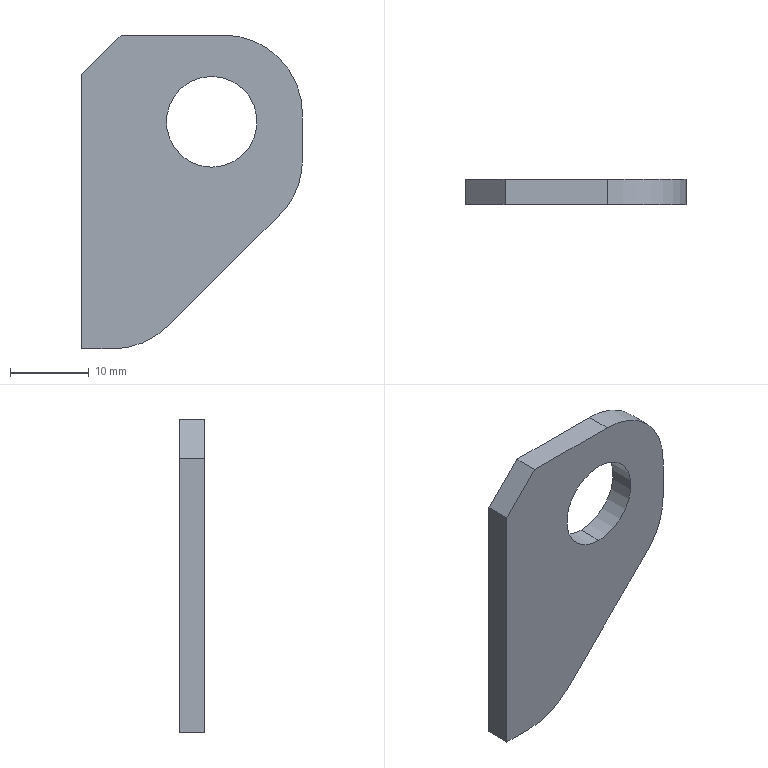Part | SolidWorks | features FlatPattern 1, SMBaseFlange 1, SheetMetal 1 | 1 solid | 13 faces | box 28 x 3.2 x 39.8 mm | volume 2478 mm3 | plane 8 | cylinder 5 | commonest cylinder face diameters 20 x3 11.5 x2
STEP:
#1=CARTESIAN_POINT('',(0.,-3.2,-5.75));
#2=VERTEX_POINT('',#1);
#3=CARTESIAN_POINT('',(0.,-3.2,5.75));
#4=VERTEX_POINT('',#3);
#5=CARTESIAN_POINT('',(0.,-3.2,0.));
#6=DIRECTION('',(0.,1.,0.));
#7=DIRECTION('',(0.,0.,1.));
#8=AXIS2_PLACEMENT_3D('',#5,#6,#7);
#9=CIRCLE('',#8,5.75);
#10=EDGE_CURVE('',#2,#4,#9,.T.);
#11=ORIENTED_EDGE('',*,*,#10,.F.);
#12=CARTESIAN_POINT('',(0.,0.,-5.75));
#13=VERTEX_POINT('',#12);
#14=CARTESIAN_POINT('',(0.,-3.2,-5.75));
#15=DIRECTION('',(0.,1.,0.));
#16=VECTOR('',#15,1000.);
#17=LINE('',#14,#16);
#18=EDGE_CURVE('',#2,#13,#17,.T.);
#19=ORIENTED_EDGE('',*,*,#18,.T.);
#20=CARTESIAN_POINT('',(0.,0.,5.75));
#21=VERTEX_POINT('',#20);
#22=CARTESIAN_POINT('',(0.,0.,0.));
#23=DIRECTION('',(0.,1.,0.));
#24=DIRECTION('',(0.,0.,1.));
#25=AXIS2_PLACEMENT_3D('',#22,#23,#24);
#26=CIRCLE('',#25,5.75);
#27=EDGE_CURVE('',#13,#21,#26,.T.);
#28=ORIENTED_EDGE('',*,*,#27,.T.);
#29=CARTESIAN_POINT('',(0.,-3.2,5.75));
#30=DIRECTION('',(0.,1.,0.));
#31=VECTOR('',#30,1000.);
#32=LINE('',#29,#31);
#33=EDGE_CURVE('',#4,#21,#32,.T.);
#34=ORIENTED_EDGE('',*,*,#33,.F.);
#35=EDGE_LOOP('',(#11,#19,#28,#34));
#36=FACE_OUTER_BOUND('',#35,.T.);
#37=CARTESIAN_POINT('',(0.,-3.2,0.));
#38=DIRECTION('',(0.,1.,0.));
#39=DIRECTION('',(0.,0.,1.));
#40=AXIS2_PLACEMENT_3D('',#37,#38,#39);
#41=CYLINDRICAL_SURFACE('',#40,5.75);
#42=ADVANCED_FACE('',(#36),#41,.F.);
#43=CARTESIAN_POINT('',(1.5,0.,11.));
#44=VERTEX_POINT('',#43);
#45=CARTESIAN_POINT('',(11.5,0.,1.));
#46=VERTEX_POINT('',#45);
#47=CARTESIAN_POINT('',(1.5,0.,1.));
#48=DIRECTION('',(0.,1.,0.));
#49=DIRECTION('',(0.,0.,1.));
#50=AXIS2_PLACEMENT_3D('',#47,#48,#49);
#51=CIRCLE('',#50,10.);
#52=EDGE_CURVE('',#44,#46,#51,.T.);
#53=ORIENTED_EDGE('',*,*,#52,.F.);
#54=CARTESIAN_POINT('',(1.5,-3.2,11.));
#55=VERTEX_POINT('',#54);
#56=CARTESIAN_POINT('',(1.5,-3.2,11.));
#57=DIRECTION('',(0.,1.,0.));
#58=VECTOR('',#57,1000.);
#59=LINE('',#56,#58);
#60=EDGE_CURVE('',#55,#44,#59,.T.);
#61=ORIENTED_EDGE('',*,*,#60,.F.);
#62=CARTESIAN_POINT('',(11.5,-3.2,1.));
#63=VERTEX_POINT('',#62);
#64=CARTESIAN_POINT('',(1.5,-3.2,1.));
#65=DIRECTION('',(0.,1.,0.));
#66=DIRECTION('',(0.,0.,1.));
#67=AXIS2_PLACEMENT_3D('',#64,#65,#66);
#68=CIRCLE('',#67,10.);
#69=EDGE_CURVE('',#55,#63,#68,.T.);
#70=ORIENTED_EDGE('',*,*,#69,.T.);
#71=CARTESIAN_POINT('',(11.5,-3.2,1.));
#72=DIRECTION('',(0.,1.,0.));
#73=VECTOR('',#72,1000.);
#74=LINE('',#71,#73);
#75=EDGE_CURVE('',#63,#46,#74,.T.);
#76=ORIENTED_EDGE('',*,*,#75,.T.);
#77=EDGE_LOOP('',(#53,#61,#70,#76));
#78=FACE_OUTER_BOUND('',#77,.T.);
#79=CARTESIAN_POINT('',(1.5,-3.2,1.));
#80=DIRECTION('',(0.,1.,0.));
#81=DIRECTION('',(0.,0.,1.));
#82=AXIS2_PLACEMENT_3D('',#79,#80,#81);
#83=CYLINDRICAL_SURFACE('',#82,10.);
#84=ADVANCED_FACE('',(#78),#83,.T.);
#85=CARTESIAN_POINT('',(-11.5,0.,11.));
#86=VERTEX_POINT('',#85);
#87=CARTESIAN_POINT('',(-11.5,0.,11.));
#88=DIRECTION('',(1.,0.,0.));
#89=VECTOR('',#88,1000.);
#90=LINE('',#87,#89);
#91=EDGE_CURVE('',#86,#44,#90,.T.);
#92=ORIENTED_EDGE('',*,*,#91,.F.);
#93=CARTESIAN_POINT('',(-11.5,-3.2,11.));
#94=VERTEX_POINT('',#93);
#95=CARTESIAN_POINT('',(-11.5,-3.2,11.));
#96=DIRECTION('',(0.,1.,0.));
#97=VECTOR('',#96,1000.);
#98=LINE('',#95,#97);
#99=EDGE_CURVE('',#94,#86,#98,.T.);
#100=ORIENTED_EDGE('',*,*,#99,.F.);
#101=CARTESIAN_POINT('',(-11.5,-3.2,11.));
#102=DIRECTION('',(1.,0.,0.));
#103=VECTOR('',#102,1000.);
#104=LINE('',#101,#103);
#105=EDGE_CURVE('',#94,#55,#104,.T.);
#106=ORIENTED_EDGE('',*,*,#105,.T.);
#107=ORIENTED_EDGE('',*,*,#60,.T.);
#108=EDGE_LOOP('',(#92,#100,#106,#107));
#109=FACE_OUTER_BOUND('',#108,.T.);
#110=CARTESIAN_POINT('',(-11.5,-3.2,11.));
#111=DIRECTION('',(0.,0.,1.));
#112=DIRECTION('',(1.,0.,0.));
#113=AXIS2_PLACEMENT_3D('',#110,#111,#112);
#114=PLANE('',#113);
#115=ADVANCED_FACE('',(#109),#114,.T.);
#116=CARTESIAN_POINT('',(-16.5,0.,6.));
#117=VERTEX_POINT('',#116);
#118=CARTESIAN_POINT('',(-16.5,0.,6.));
#119=DIRECTION('',(0.7071,0.,0.7071));
#120=VECTOR('',#119,1000.);
#121=LINE('',#118,#120);
#122=EDGE_CURVE('',#117,#86,#121,.T.);
#123=ORIENTED_EDGE('',*,*,#122,.F.);
#124=CARTESIAN_POINT('',(-16.5,-3.2,6.));
#125=VERTEX_POINT('',#124);
#126=CARTESIAN_POINT('',(-16.5,-3.2,6.));
#127=DIRECTION('',(0.,1.,0.));
#128=VECTOR('',#127,1000.);
#129=LINE('',#126,#128);
#130=EDGE_CURVE('',#125,#117,#129,.T.);
#131=ORIENTED_EDGE('',*,*,#130,.F.);
#132=CARTESIAN_POINT('',(-16.5,-3.2,6.));
#133=DIRECTION('',(0.7071,0.,0.7071));
#134=VECTOR('',#133,1000.);
#135=LINE('',#132,#134);
#136=EDGE_CURVE('',#125,#94,#135,.T.);
#137=ORIENTED_EDGE('',*,*,#136,.T.);
#138=ORIENTED_EDGE('',*,*,#99,.T.);
#139=EDGE_LOOP('',(#123,#131,#137,#138));
#140=FACE_OUTER_BOUND('',#139,.T.);
#141=CARTESIAN_POINT('',(-16.5,-3.2,6.));
#142=DIRECTION('',(-0.7071,0.,0.7071));
#143=DIRECTION('',(0.7071,0.,0.7071));
#144=AXIS2_PLACEMENT_3D('',#141,#142,#143);
#145=PLANE('',#144);
#146=ADVANCED_FACE('',(#140),#145,.T.);
#147=CARTESIAN_POINT('',(-16.5,0.,-28.8));
#148=VERTEX_POINT('',#147);
#149=CARTESIAN_POINT('',(-16.5,0.,-28.8));
#150=DIRECTION('',(0.,0.,1.));
#151=VECTOR('',#150,1000.);
#152=LINE('',#149,#151);
#153=EDGE_CURVE('',#148,#117,#152,.T.);
#154=ORIENTED_EDGE('',*,*,#153,.F.);
#155=CARTESIAN_POINT('',(-16.5,-3.2,-28.8));
#156=VERTEX_POINT('',#155);
#157=CARTESIAN_POINT('',(-16.5,-3.2,-28.8));
#158=DIRECTION('',(0.,1.,0.));
#159=VECTOR('',#158,1000.);
#160=LINE('',#157,#159);
#161=EDGE_CURVE('',#156,#148,#160,.T.);
#162=ORIENTED_EDGE('',*,*,#161,.F.);
#163=CARTESIAN_POINT('',(-16.5,-3.2,-28.8));
#164=DIRECTION('',(0.,0.,1.));
#165=VECTOR('',#164,1000.);
#166=LINE('',#163,#165);
#167=EDGE_CURVE('',#156,#125,#166,.T.);
#168=ORIENTED_EDGE('',*,*,#167,.T.);
#169=ORIENTED_EDGE('',*,*,#130,.T.);
#170=EDGE_LOOP('',(#154,#162,#168,#169));
#171=FACE_OUTER_BOUND('',#170,.T.);
#172=CARTESIAN_POINT('',(-16.5,-3.2,-28.8));
#173=DIRECTION('',(-1.,0.,0.));
#174=DIRECTION('',(0.,0.,1.));
#175=AXIS2_PLACEMENT_3D('',#172,#173,#174);
#176=PLANE('',#175);
#177=ADVANCED_FACE('',(#171),#176,.T.);
#178=CARTESIAN_POINT('',(-12.613,0.,-28.8));
#179=VERTEX_POINT('',#178);
#180=CARTESIAN_POINT('',(-12.613,0.,-28.8));
#181=DIRECTION('',(-1.,0.,0.));
#182=VECTOR('',#181,1000.);
#183=LINE('',#180,#182);
#184=EDGE_CURVE('',#179,#148,#183,.T.);
#185=ORIENTED_EDGE('',*,*,#184,.F.);
#186=CARTESIAN_POINT('',(-12.613,-3.2,-28.8));
#187=VERTEX_POINT('',#186);
#188=CARTESIAN_POINT('',(-12.613,-3.2,-28.8));
#189=DIRECTION('',(0.,1.,0.));
#190=VECTOR('',#189,1000.);
#191=LINE('',#188,#190);
#192=EDGE_CURVE('',#187,#179,#191,.T.);
#193=ORIENTED_EDGE('',*,*,#192,.F.);
#194=CARTESIAN_POINT('',(-12.613,-3.2,-28.8));
#195=DIRECTION('',(-1.,0.,0.));
#196=VECTOR('',#195,1000.);
#197=LINE('',#194,#196);
#198=EDGE_CURVE('',#187,#156,#197,.T.);
#199=ORIENTED_EDGE('',*,*,#198,.T.);
#200=ORIENTED_EDGE('',*,*,#161,.T.);
#201=EDGE_LOOP('',(#185,#193,#199,#200));
#202=FACE_OUTER_BOUND('',#201,.T.);
#203=CARTESIAN_POINT('',(-12.613,-3.2,-28.8));
#204=DIRECTION('',(0.,0.,-1.));
#205=DIRECTION('',(-1.,0.,0.));
#206=AXIS2_PLACEMENT_3D('',#203,#204,#205);
#207=PLANE('',#206);
#208=ADVANCED_FACE('',(#202),#207,.T.);
#209=CARTESIAN_POINT('',(-5.577,0.,-25.907));
#210=VERTEX_POINT('',#209);
#211=CARTESIAN_POINT('',(-12.613,0.,-18.8));
#212=DIRECTION('',(0.,1.,0.));
#213=DIRECTION('',(0.,0.,1.));
#214=AXIS2_PLACEMENT_3D('',#211,#212,#213);
#215=CIRCLE('',#214,10.);
#216=EDGE_CURVE('',#210,#179,#215,.T.);
#217=ORIENTED_EDGE('',*,*,#216,.F.);
#218=CARTESIAN_POINT('',(-5.577,-3.2,-25.907));
#219=VERTEX_POINT('',#218);
#220=CARTESIAN_POINT('',(-5.577,-3.2,-25.907));
#221=DIRECTION('',(0.,1.,0.));
#222=VECTOR('',#221,1000.);
#223=LINE('',#220,#222);
#224=EDGE_CURVE('',#219,#210,#223,.T.);
#225=ORIENTED_EDGE('',*,*,#224,.F.);
#226=CARTESIAN_POINT('',(-12.613,-3.2,-18.8));
#227=DIRECTION('',(0.,1.,0.));
#228=DIRECTION('',(0.,0.,1.));
#229=AXIS2_PLACEMENT_3D('',#226,#227,#228);
#230=CIRCLE('',#229,10.);
#231=EDGE_CURVE('',#219,#187,#230,.T.);
#232=ORIENTED_EDGE('',*,*,#231,.T.);
#233=ORIENTED_EDGE('',*,*,#192,.T.);
#234=EDGE_LOOP('',(#217,#225,#232,#233));
#235=FACE_OUTER_BOUND('',#234,.T.);
#236=CARTESIAN_POINT('',(-12.613,-3.2,-18.8));
#237=DIRECTION('',(0.,1.,0.));
#238=DIRECTION('',(0.,0.,1.));
#239=AXIS2_PLACEMENT_3D('',#236,#237,#238);
#240=CYLINDRICAL_SURFACE('',#239,10.);
#241=ADVANCED_FACE('',(#235),#240,.T.);
#242=CARTESIAN_POINT('',(8.535,0.,-11.935));
#243=VERTEX_POINT('',#242);
#244=CARTESIAN_POINT('',(8.535,0.,-11.935));
#245=DIRECTION('',(-0.7107,0.,-0.7035));
#246=VECTOR('',#245,1000.);
#247=LINE('',#244,#246);
#248=EDGE_CURVE('',#243,#210,#247,.T.);
#249=ORIENTED_EDGE('',*,*,#248,.F.);
#250=CARTESIAN_POINT('',(8.535,-3.2,-11.935));
#251=VERTEX_POINT('',#250);
#252=CARTESIAN_POINT('',(8.535,-3.2,-11.935));
#253=DIRECTION('',(0.,1.,0.));
#254=VECTOR('',#253,1000.);
#255=LINE('',#252,#254);
#256=EDGE_CURVE('',#251,#243,#255,.T.);
#257=ORIENTED_EDGE('',*,*,#256,.F.);
#258=CARTESIAN_POINT('',(8.535,-3.2,-11.935));
#259=DIRECTION('',(-0.7107,0.,-0.7035));
#260=VECTOR('',#259,1000.);
#261=LINE('',#258,#260);
#262=EDGE_CURVE('',#251,#219,#261,.T.);
#263=ORIENTED_EDGE('',*,*,#262,.T.);
#264=ORIENTED_EDGE('',*,*,#224,.T.);
#265=EDGE_LOOP('',(#249,#257,#263,#264));
#266=FACE_OUTER_BOUND('',#265,.T.);
#267=CARTESIAN_POINT('',(8.535,-3.2,-11.935));
#268=DIRECTION('',(0.7035,0.,-0.7107));
#269=DIRECTION('',(-0.7107,0.,-0.7035));
#270=AXIS2_PLACEMENT_3D('',#267,#268,#269);
#271=PLANE('',#270);
#272=ADVANCED_FACE('',(#266),#271,.T.);
#273=CARTESIAN_POINT('',(11.5,0.,-4.828));
#274=VERTEX_POINT('',#273);
#275=CARTESIAN_POINT('',(1.5,0.,-4.828));
#276=DIRECTION('',(0.,1.,0.));
#277=DIRECTION('',(0.,0.,1.));
#278=AXIS2_PLACEMENT_3D('',#275,#276,#277);
#279=CIRCLE('',#278,10.);
#280=EDGE_CURVE('',#274,#243,#279,.T.);
#281=ORIENTED_EDGE('',*,*,#280,.F.);
#282=CARTESIAN_POINT('',(11.5,-3.2,-4.828));
#283=VERTEX_POINT('',#282);
#284=CARTESIAN_POINT('',(11.5,-3.2,-4.828));
#285=DIRECTION('',(0.,1.,0.));
#286=VECTOR('',#285,1000.);
#287=LINE('',#284,#286);
#288=EDGE_CURVE('',#283,#274,#287,.T.);
#289=ORIENTED_EDGE('',*,*,#288,.F.);
#290=CARTESIAN_POINT('',(1.5,-3.2,-4.828));
#291=DIRECTION('',(0.,1.,0.));
#292=DIRECTION('',(0.,0.,1.));
#293=AXIS2_PLACEMENT_3D('',#290,#291,#292);
#294=CIRCLE('',#293,10.);
#295=EDGE_CURVE('',#283,#251,#294,.T.);
#296=ORIENTED_EDGE('',*,*,#295,.T.);
#297=ORIENTED_EDGE('',*,*,#256,.T.);
#298=EDGE_LOOP('',(#281,#289,#296,#297));
#299=FACE_OUTER_BOUND('',#298,.T.);
#300=CARTESIAN_POINT('',(1.5,-3.2,-4.828));
#301=DIRECTION('',(0.,1.,0.));
#302=DIRECTION('',(0.,0.,1.));
#303=AXIS2_PLACEMENT_3D('',#300,#301,#302);
#304=CYLINDRICAL_SURFACE('',#303,10.);
#305=ADVANCED_FACE('',(#299),#304,.T.);
#306=CARTESIAN_POINT('',(11.5,0.,1.));
#307=DIRECTION('',(0.,0.,-1.));
#308=VECTOR('',#307,1000.);
#309=LINE('',#306,#308);
#310=EDGE_CURVE('',#46,#274,#309,.T.);
#311=ORIENTED_EDGE('',*,*,#310,.F.);
#312=ORIENTED_EDGE('',*,*,#75,.F.);
#313=CARTESIAN_POINT('',(11.5,-3.2,1.));
#314=DIRECTION('',(0.,0.,-1.));
#315=VECTOR('',#314,1000.);
#316=LINE('',#313,#315);
#317=EDGE_CURVE('',#63,#283,#316,.T.);
#318=ORIENTED_EDGE('',*,*,#317,.T.);
#319=ORIENTED_EDGE('',*,*,#288,.T.);
#320=EDGE_LOOP('',(#311,#312,#318,#319));
#321=FACE_OUTER_BOUND('',#320,.T.);
#322=CARTESIAN_POINT('',(11.5,-3.2,1.));
#323=DIRECTION('',(1.,0.,0.));
#324=DIRECTION('',(0.,0.,-1.));
#325=AXIS2_PLACEMENT_3D('',#322,#323,#324);
#326=PLANE('',#325);
#327=ADVANCED_FACE('',(#321),#326,.T.);
#328=CARTESIAN_POINT('',(0.,-3.2,0.));
#329=DIRECTION('',(0.,1.,0.));
#330=DIRECTION('',(0.,0.,1.));
#331=AXIS2_PLACEMENT_3D('',#328,#329,#330);
#332=CIRCLE('',#331,5.75);
#333=EDGE_CURVE('',#4,#2,#332,.T.);
#334=ORIENTED_EDGE('',*,*,#333,.T.);
#335=ORIENTED_EDGE('',*,*,#10,.T.);
#336=EDGE_LOOP('',(#334,#335));
#337=FACE_BOUND('',#336,.T.);
#338=ORIENTED_EDGE('',*,*,#69,.F.);
#339=ORIENTED_EDGE('',*,*,#105,.F.);
#340=ORIENTED_EDGE('',*,*,#136,.F.);
#341=ORIENTED_EDGE('',*,*,#167,.F.);
#342=ORIENTED_EDGE('',*,*,#198,.F.);
#343=ORIENTED_EDGE('',*,*,#231,.F.);
#344=ORIENTED_EDGE('',*,*,#262,.F.);
#345=ORIENTED_EDGE('',*,*,#295,.F.);
#346=ORIENTED_EDGE('',*,*,#317,.F.);
#347=EDGE_LOOP('',(#338,#339,#340,#341,#342,#343,#344,#345,#346));
#348=FACE_OUTER_BOUND('',#347,.T.);
#349=CARTESIAN_POINT('',(1.5,-3.2,1.));
#350=DIRECTION('',(0.,1.,0.));
#351=DIRECTION('',(0.,0.,1.));
#352=AXIS2_PLACEMENT_3D('',#349,#350,#351);
#353=PLANE('',#352);
#354=ADVANCED_FACE('',(#337,#348),#353,.F.);
#355=CARTESIAN_POINT('',(0.,0.,0.));
#356=DIRECTION('',(0.,1.,0.));
#357=DIRECTION('',(0.,0.,1.));
#358=AXIS2_PLACEMENT_3D('',#355,#356,#357);
#359=CIRCLE('',#358,5.75);
#360=EDGE_CURVE('',#21,#13,#359,.T.);
#361=ORIENTED_EDGE('',*,*,#360,.F.);
#362=ORIENTED_EDGE('',*,*,#27,.F.);
#363=EDGE_LOOP('',(#361,#362));
#364=FACE_BOUND('',#363,.T.);
#365=ORIENTED_EDGE('',*,*,#52,.T.);
#366=ORIENTED_EDGE('',*,*,#310,.T.);
#367=ORIENTED_EDGE('',*,*,#280,.T.);
#368=ORIENTED_EDGE('',*,*,#248,.T.);
#369=ORIENTED_EDGE('',*,*,#216,.T.);
#370=ORIENTED_EDGE('',*,*,#184,.T.);
#371=ORIENTED_EDGE('',*,*,#153,.T.);
#372=ORIENTED_EDGE('',*,*,#122,.T.);
#373=ORIENTED_EDGE('',*,*,#91,.T.);
#374=EDGE_LOOP('',(#365,#366,#367,#368,#369,#370,#371,#372,#373));
#375=FACE_OUTER_BOUND('',#374,.T.);
#376=CARTESIAN_POINT('',(1.5,0.,1.));
#377=DIRECTION('',(0.,1.,0.));
#378=DIRECTION('',(0.,0.,1.));
#379=AXIS2_PLACEMENT_3D('',#376,#377,#378);
#380=PLANE('',#379);
#381=ADVANCED_FACE('',(#364,#375),#380,.T.);
#382=ORIENTED_EDGE('',*,*,#18,.F.);
#383=ORIENTED_EDGE('',*,*,#333,.F.);
#384=ORIENTED_EDGE('',*,*,#33,.T.);
#385=ORIENTED_EDGE('',*,*,#360,.T.);
#386=EDGE_LOOP('',(#382,#383,#384,#385));
#387=FACE_OUTER_BOUND('',#386,.T.);
#388=CARTESIAN_POINT('',(0.,-3.2,0.));
#389=DIRECTION('',(0.,1.,0.));
#390=DIRECTION('',(0.,0.,1.));
#391=AXIS2_PLACEMENT_3D('',#388,#389,#390);
#392=CYLINDRICAL_SURFACE('',#391,5.75);
#393=ADVANCED_FACE('',(#387),#392,.F.);
#394=CLOSED_SHELL('',(#42,#84,#115,#146,#177,#208,#241,#272,#305,#327,#354,#381,#393));
#395=MANIFOLD_SOLID_BREP('',#394);
#396=CARTESIAN_POINT('',(0.,0.,0.));
#397=DIRECTION('',(0.,0.,1.));
#398=DIRECTION('',(1.,0.,0.));
#399=AXIS2_PLACEMENT_3D('',#396,#397,#398);
#400=(LENGTH_UNIT()NAMED_UNIT(*)SI_UNIT(.MILLI.,.METRE.));
#401=UNCERTAINTY_MEASURE_WITH_UNIT(LENGTH_MEASURE(0.00001),#400,'','');
#402=(NAMED_UNIT(*)PLANE_ANGLE_UNIT()SI_UNIT($,.RADIAN.));
#403=(NAMED_UNIT(*)SI_UNIT($,.STERADIAN.)SOLID_ANGLE_UNIT());
#404=(GEOMETRIC_REPRESENTATION_CONTEXT(3)GLOBAL_UNCERTAINTY_ASSIGNED_CONTEXT((#401))GLOBAL_UNIT_ASSIGNED_CONTEXT((#400,#402,#403))REPRESENTATION_CONTEXT('',''));
#405=ADVANCED_BREP_SHAPE_REPRESENTATION('',(#395,#399),#404);